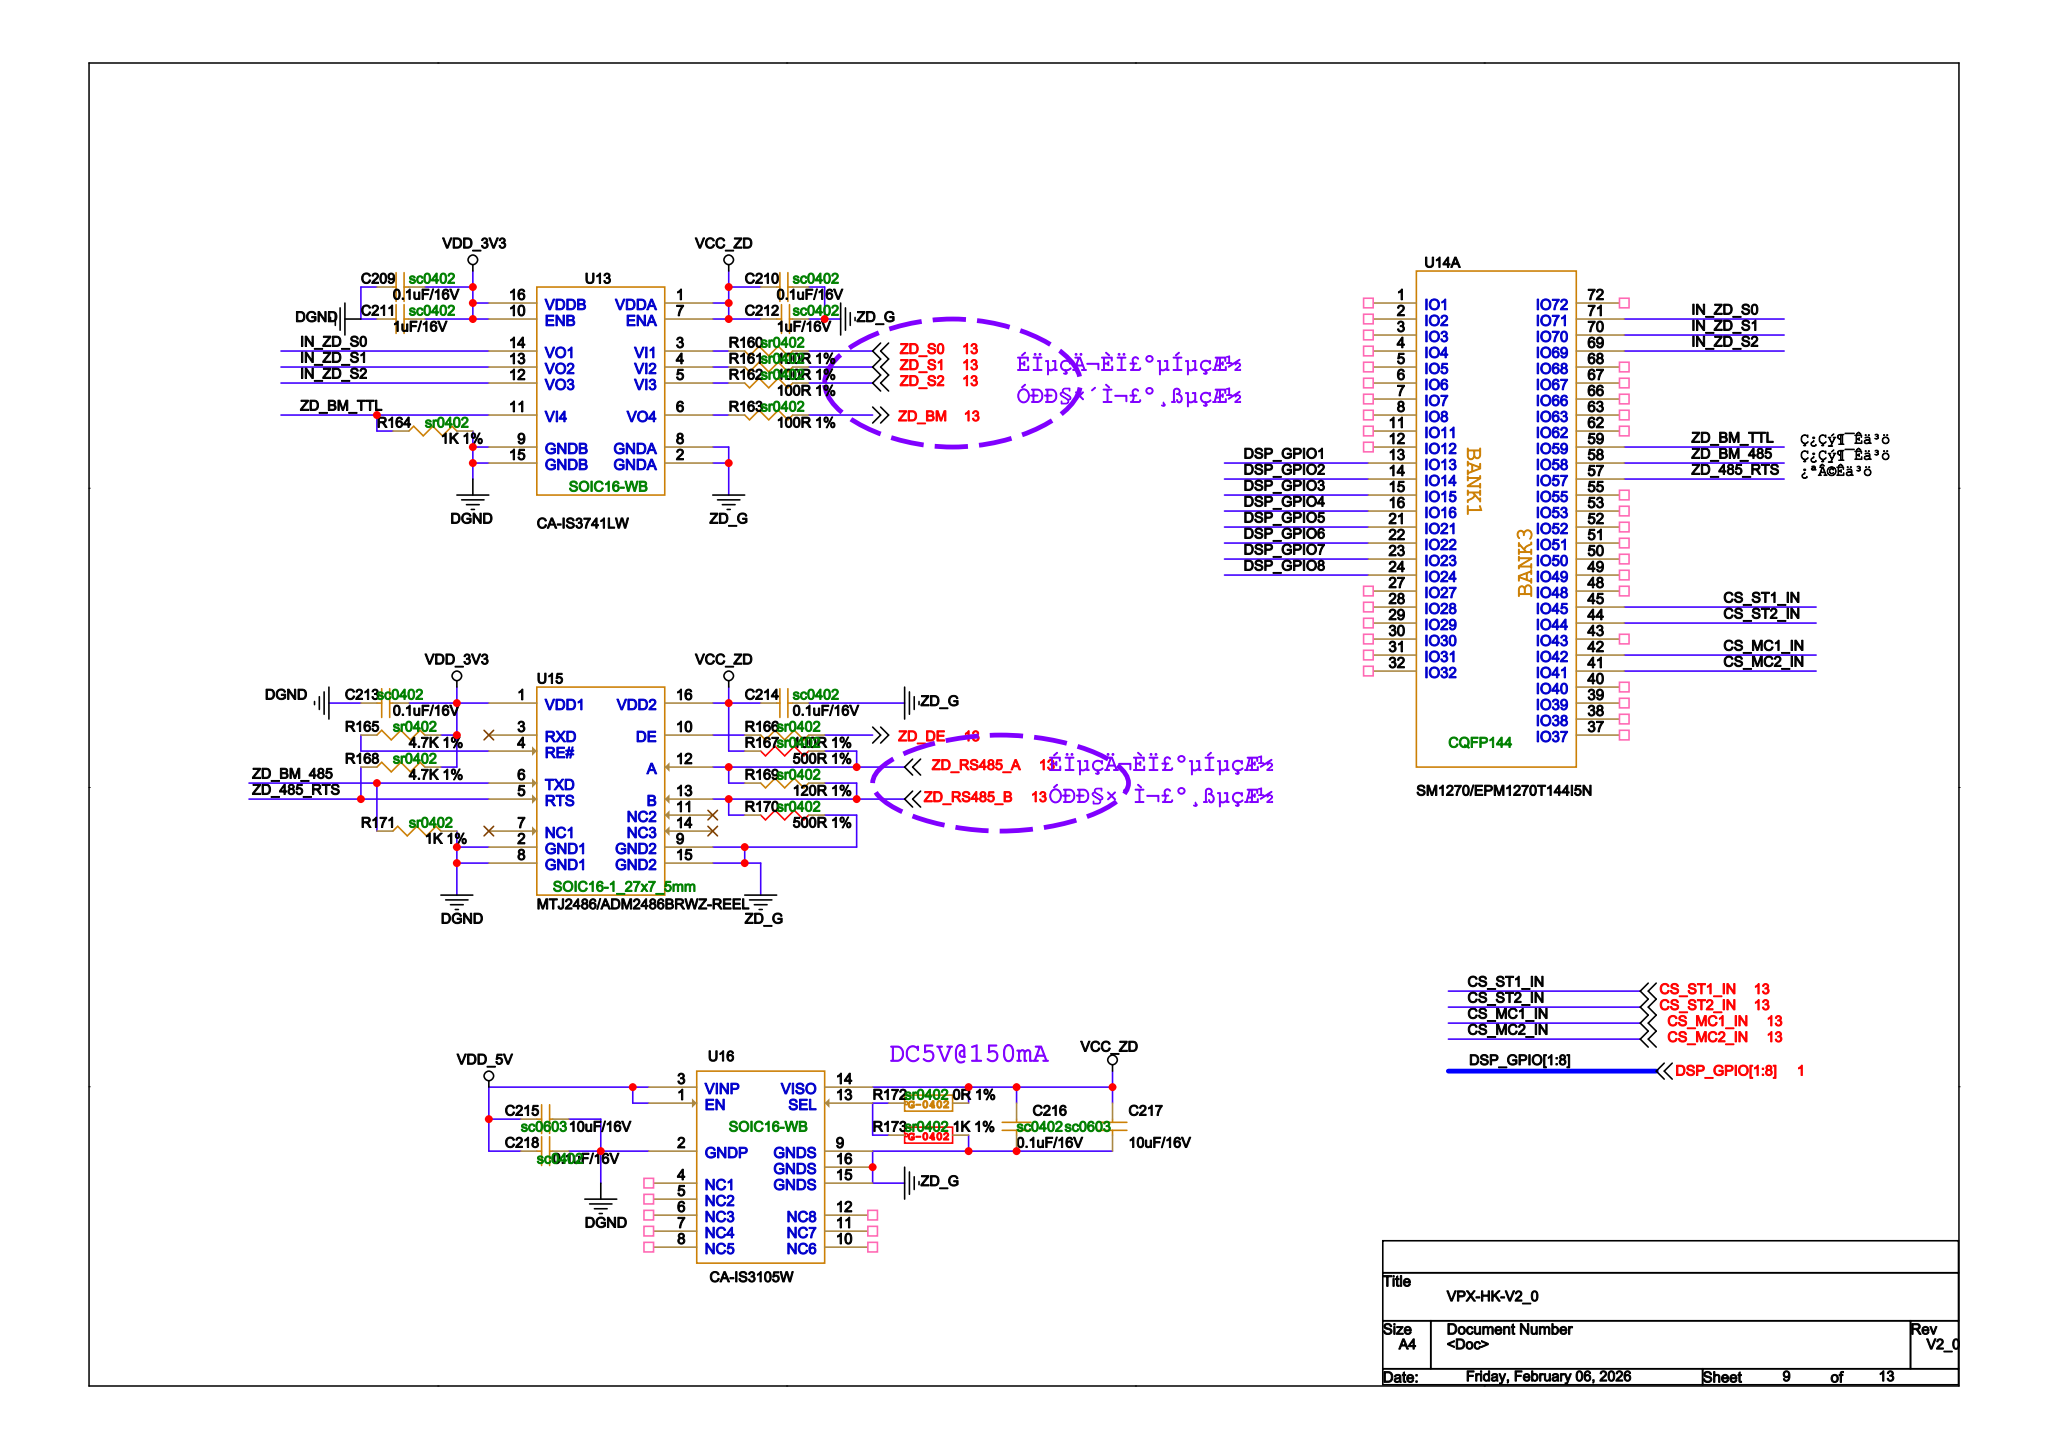Circuit board | Cadence Allegro | 598 parts | 541 nets | one sheet of the schematic
Parts on this sheet (reference | value | footprint):
C209 | 0.1uF/16V | SC0402
C210 | 0.1uF/16V | SC0402
C211 | 1uF/16V | SC0402
C212 | 1uF/16V | SC0402
C213 | 0.1uF/16V | SC0402
C214 | 0.1uF/16V | SC0402
C215 | 10uF/16V | SC0603
C216 | 0.1uF/16V | SC0402
C217 | 10uF/16V | SC0603
C218 | 0.1uF/16V | SC0402
R160 | 100R 1% | SR0402
R161 | 100R 1% | SR0402
R162 | 100R 1% | SR0402
R163 | 100R 1% | SR0402
R164 | 1K 1% | SR0402
R165 | 4.7K 1% | SR0402
R166 | 100R 1% | SR0402
R167 | 500R 1% | SR0402
R168 | 4.7K 1% | SR0402
R169 | 120R 1% | SR0402
R170 | 500R 1% | SR0402
R171 | 1K 1% | SR0402
U13 | CA-IS3741LW | SOIC16-WB
U14 | SM1270/EPM1270T144I5N | CQFP144
U15 | MTJ2486/ADM2486BRWZ-REEL | SOIC16-1_27X7_5MM
U16 | CA-IS3105W | SOIC16-WB
Nets of these parts (net: part-pin ...):
DGND: C209-1 C211-1 C213-2 C215-1 C218-1 R164-2 R171-2 U13-9 U13-15 U15-2 U15-8 U16-2 U14-10
VDD_5V: C215-2 C218-2 U16-1 U16-3
DSP_GPIO1: U14-13
DSP_GPIO2: U14-14
DSP_GPIO3: U14-15
DSP_GPIO4: U14-16
DSP_GPIO5: U14-21
DSP_GPIO6: U14-22
DSP_GPIO7: U14-23
DSP_GPIO8: U14-24
CS_MC2_IN: U14-41
CS_MC1_IN: U14-42
CS_ST2_IN: U14-44
CS_ST1_IN: U14-45
ZD_485_RTS: R168-1 U15-5 U14-57
ZD_BM_485: R171-1 U15-6 U14-58
ZD_BM_TTL: R164-1 U13-11 U14-59
IN_ZD_S2: U13-12 U14-69
IN_ZD_S1: U13-13 U14-70
IN_ZD_S0: U13-14 U14-71
ZD_RS485_A: R167-1 R169-2 U15-12
ZD_RS485_B: R169-1 R170-2 U15-13
N33596289: R166-2 U15-10
ZD_G: C210-2 C212-1 C214-2 C216-2 C217-2 R170-1 U13-2 U13-8 U15-9 U15-15 U16-9 U16-15 U16-16
N33594812: R165-1 U15-4
VDD_3V3: C209-2 C211-2 C213-1 R165-2 R168-2 U13-10 U13-16 U15-1
VCC_ZD: C210-1 C212-2 C214-1 C216-1 C217-1 R167-2 U13-1 U13-7 U15-16 U16-14
N33499596: U16-13
ZD_BM: R163-1
ZD_S1: R161-1
ZD_S2: R162-1
ZD_S0: R160-1
ZD_DE: R166-1
N33506634: R163-2 U13-6
N33587343: R160-2 U13-3
N33506632: R161-2 U13-4
N33587357: R162-2 U13-5